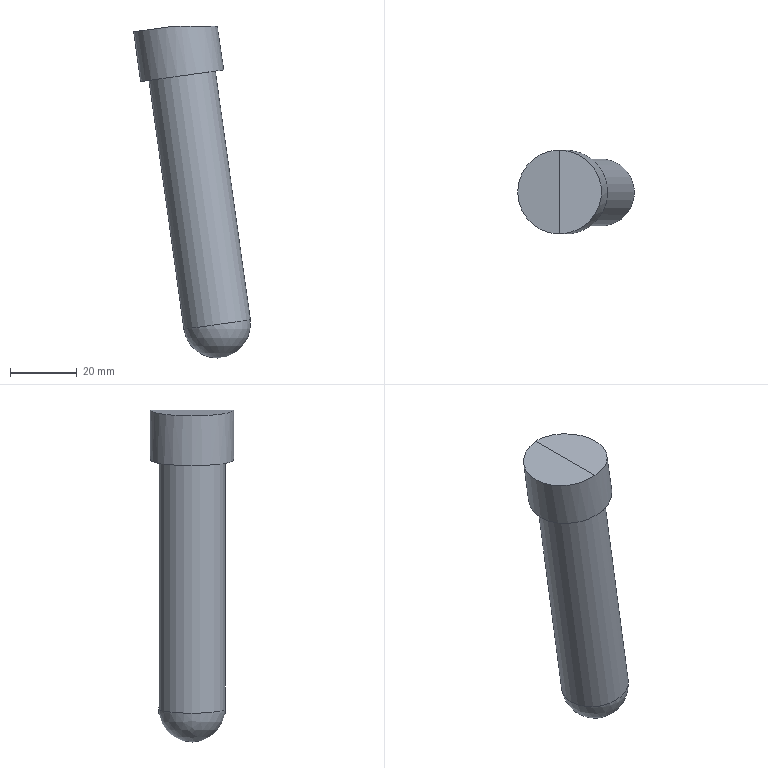Part | STEP file | P011002S002-011 | 1 solid | 6 faces | box 34.904 x 25 x 99.124 mm | volume 32836 mm3 | plane 3 | cylinder 2 | sphere 1 | commonest cylinder face diameters 20 x1 25 x1
STEP:
#1=CARTESIAN_POINT('',(0.,0.,0.));
#2=DIRECTION('',(0.,0.,1.));
#3=DIRECTION('',(1.,0.,0.));
#4=AXIS2_PLACEMENT_3D('',#1,#2,#3);
#5=CARTESIAN_POINT('',(193.,47.5,61.));
#6=VERTEX_POINT('',#5);
#7=CARTESIAN_POINT('',(193.,72.5,61.));
#8=VERTEX_POINT('',#7);
#9=CARTESIAN_POINT('',(193.,60.,61.));
#10=DIRECTION('',(0.,1.,0.));
#11=VECTOR('',#10,1.);
#12=LINE('',#9,#11);
#13=CARTESIAN_POINT('',(193.,60.,61.));
#14=DIRECTION('',(0.1392,0.,-0.9903));
#15=DIRECTION('',(0.9903,0.,0.1392));
#16=AXIS2_PLACEMENT_3D('',#13,#14,#15);
#17=PLANE('',#16);
#18=CARTESIAN_POINT('',(0.,0.));
#19=DIRECTION('',(0.,-1.));
#20=VECTOR('',#19,1.);
#21=LINE('',#18,#20);
#22=(GEOMETRIC_REPRESENTATION_CONTEXT(2)PARAMETRIC_REPRESENTATION_CONTEXT()REPRESENTATION_CONTEXT('',''));
#23=DEFINITIONAL_REPRESENTATION('',(#21),#22);
#24=PCURVE('',#17,#23);
#25=CARTESIAN_POINT('',(250.,10.,61.));
#26=DIRECTION('',(0.,0.,1.));
#27=DIRECTION('',(-1.,0.,0.));
#28=AXIS2_PLACEMENT_3D('',#25,#26,#27);
#29=PLANE('',#28);
#30=CARTESIAN_POINT('',(57.,-50.));
#31=DIRECTION('',(0.,-1.));
#32=VECTOR('',#31,1.);
#33=LINE('',#30,#32);
#34=(GEOMETRIC_REPRESENTATION_CONTEXT(2)PARAMETRIC_REPRESENTATION_CONTEXT()REPRESENTATION_CONTEXT('',''));
#35=DEFINITIONAL_REPRESENTATION('',(#33),#34);
#36=PCURVE('',#29,#35);
#37=SURFACE_CURVE('',#12,(#24,#36),.PCURVE_S1.);
#38=EDGE_CURVE('',#6,#8,#37,.T.);
#39=ORIENTED_EDGE('',*,*,#38,.T.);
#40=CARTESIAN_POINT('',(180.622,60.,59.26));
#41=VERTEX_POINT('',#40);
#42=CARTESIAN_POINT('',(193.,60.,61.));
#43=DIRECTION('',(-0.1392,0.,0.9903));
#44=DIRECTION('',(0.9903,0.,0.1392));
#45=AXIS2_PLACEMENT_3D('',#42,#43,#44);
#46=CIRCLE('',#45,12.5);
#47=CARTESIAN_POINT('',(12.5,0.));
#48=CARTESIAN_POINT('',(12.5,-21.651));
#49=CARTESIAN_POINT('',(-6.25,-10.825));
#50=CARTESIAN_POINT('',(-25.,0.));
#51=CARTESIAN_POINT('',(-6.25,10.825));
#52=CARTESIAN_POINT('',(12.5,21.651));
#53=CARTESIAN_POINT('',(12.5,0.));
#54=(BOUNDED_CURVE()B_SPLINE_CURVE(2,(#47,#48,#49,#50,#51,#52,#53),.UNSPECIFIED.,.T.,.F.)B_SPLINE_CURVE_WITH_KNOTS((1,2,2,2,2,1),(-2.094,0.,2.094,4.189,6.283,8.378),.UNSPECIFIED.)CURVE()GEOMETRIC_REPRESENTATION_ITEM()RATIONAL_B_SPLINE_CURVE((1.,0.5,1.,0.5,1.,0.5,1.))REPRESENTATION_ITEM(''));
#55=(GEOMETRIC_REPRESENTATION_CONTEXT(2)PARAMETRIC_REPRESENTATION_CONTEXT()REPRESENTATION_CONTEXT('',''));
#56=DEFINITIONAL_REPRESENTATION('',(#54),#55);
#57=PCURVE('',#17,#56);
#58=CARTESIAN_POINT('',(223.831,60.,-158.375));
#59=DIRECTION('',(-0.1392,0.,0.9903));
#60=DIRECTION('',(-0.9903,0.,-0.1392));
#61=AXIS2_PLACEMENT_3D('',#58,#59,#60);
#62=CYLINDRICAL_SURFACE('',#61,12.5);
#63=CARTESIAN_POINT('',(3.142,221.531));
#64=DIRECTION('',(1.,0.));
#65=VECTOR('',#64,1.);
#66=LINE('',#63,#65);
#67=(GEOMETRIC_REPRESENTATION_CONTEXT(2)PARAMETRIC_REPRESENTATION_CONTEXT()REPRESENTATION_CONTEXT('',''));
#68=DEFINITIONAL_REPRESENTATION('',(#66),#67);
#69=PCURVE('',#62,#68);
#70=SURFACE_CURVE('',#46,(#57,#69),.PCURVE_S1.);
#71=EDGE_CURVE('',#8,#41,#70,.T.);
#72=ORIENTED_EDGE('',*,*,#71,.T.);
#73=CARTESIAN_POINT('',(193.,60.,61.));
#74=DIRECTION('',(-0.1392,0.,0.9903));
#75=DIRECTION('',(0.9903,0.,0.1392));
#76=AXIS2_PLACEMENT_3D('',#73,#74,#75);
#77=CIRCLE('',#76,12.5);
#78=CARTESIAN_POINT('',(12.5,0.));
#79=CARTESIAN_POINT('',(12.5,-21.651));
#80=CARTESIAN_POINT('',(-6.25,-10.825));
#81=CARTESIAN_POINT('',(-25.,0.));
#82=CARTESIAN_POINT('',(-6.25,10.825));
#83=CARTESIAN_POINT('',(12.5,21.651));
#84=CARTESIAN_POINT('',(12.5,0.));
#85=(BOUNDED_CURVE()B_SPLINE_CURVE(2,(#78,#79,#80,#81,#82,#83,#84),.UNSPECIFIED.,.T.,.F.)B_SPLINE_CURVE_WITH_KNOTS((1,2,2,2,2,1),(-2.094,0.,2.094,4.189,6.283,8.378),.UNSPECIFIED.)CURVE()GEOMETRIC_REPRESENTATION_ITEM()RATIONAL_B_SPLINE_CURVE((1.,0.5,1.,0.5,1.,0.5,1.))REPRESENTATION_ITEM(''));
#86=(GEOMETRIC_REPRESENTATION_CONTEXT(2)PARAMETRIC_REPRESENTATION_CONTEXT()REPRESENTATION_CONTEXT('',''));
#87=DEFINITIONAL_REPRESENTATION('',(#85),#86);
#88=PCURVE('',#17,#87);
#89=CARTESIAN_POINT('',(-3.142,221.531));
#90=DIRECTION('',(1.,0.));
#91=VECTOR('',#90,1.);
#92=LINE('',#89,#91);
#93=(GEOMETRIC_REPRESENTATION_CONTEXT(2)PARAMETRIC_REPRESENTATION_CONTEXT()REPRESENTATION_CONTEXT('',''));
#94=DEFINITIONAL_REPRESENTATION('',(#92),#93);
#95=PCURVE('',#62,#94);
#96=SURFACE_CURVE('',#77,(#88,#95),.PCURVE_S1.);
#97=EDGE_CURVE('',#41,#6,#96,.T.);
#98=ORIENTED_EDGE('',*,*,#97,.T.);
#99=EDGE_LOOP('',(#39,#72,#98));
#100=FACE_BOUND('',#99,.T.);
#101=ADVANCED_FACE('',(#100),#17,.F.);
#102=CARTESIAN_POINT('',(182.709,60.,44.406));
#103=VERTEX_POINT('',#102);
#104=CARTESIAN_POINT('',(195.088,60.,46.146));
#105=DIRECTION('',(0.1392,0.,-0.9903));
#106=DIRECTION('',(-0.9903,0.,-0.1392));
#107=AXIS2_PLACEMENT_3D('',#104,#105,#106);
#108=CIRCLE('',#107,12.5);
#109=CARTESIAN_POINT('',(6.283,206.531));
#110=DIRECTION('',(-1.,0.));
#111=VECTOR('',#110,1.);
#112=LINE('',#109,#111);
#113=(GEOMETRIC_REPRESENTATION_CONTEXT(2)PARAMETRIC_REPRESENTATION_CONTEXT()REPRESENTATION_CONTEXT('',''));
#114=DEFINITIONAL_REPRESENTATION('',(#112),#113);
#115=PCURVE('',#62,#114);
#116=CARTESIAN_POINT('',(195.088,105.,46.146));
#117=DIRECTION('',(-0.1392,0.,0.9903));
#118=DIRECTION('',(-0.9903,0.,-0.1392));
#119=AXIS2_PLACEMENT_3D('',#116,#117,#118);
#120=PLANE('',#119);
#121=CARTESIAN_POINT('',(12.5,45.));
#122=CARTESIAN_POINT('',(12.5,23.349));
#123=CARTESIAN_POINT('',(-6.25,34.175));
#124=CARTESIAN_POINT('',(-25.,45.));
#125=CARTESIAN_POINT('',(-6.25,55.825));
#126=CARTESIAN_POINT('',(12.5,66.651));
#127=CARTESIAN_POINT('',(12.5,45.));
#128=(BOUNDED_CURVE()B_SPLINE_CURVE(2,(#121,#122,#123,#124,#125,#126,#127),.UNSPECIFIED.,.T.,.F.)B_SPLINE_CURVE_WITH_KNOTS((1,2,2,2,2,1),(-2.094,0.,2.094,4.189,6.283,8.378),.UNSPECIFIED.)CURVE()GEOMETRIC_REPRESENTATION_ITEM()RATIONAL_B_SPLINE_CURVE((1.,0.5,1.,0.5,1.,0.5,1.))REPRESENTATION_ITEM(''));
#129=(GEOMETRIC_REPRESENTATION_CONTEXT(2)PARAMETRIC_REPRESENTATION_CONTEXT()REPRESENTATION_CONTEXT('',''));
#130=DEFINITIONAL_REPRESENTATION('',(#128),#129);
#131=PCURVE('',#120,#130);
#132=SURFACE_CURVE('',#108,(#115,#131),.PCURVE_S1.);
#133=EDGE_CURVE('',#103,#103,#132,.T.);
#134=ORIENTED_EDGE('',*,*,#133,.F.);
#135=CARTESIAN_POINT('',(182.709,60.,44.406));
#136=CARTESIAN_POINT('',(180.622,60.,59.26));
#137=B_SPLINE_CURVE_WITH_KNOTS('',1,(#135,#136),.UNSPECIFIED.,.F.,.F.,(2,2),(206.531,221.531),.PIECEWISE_BEZIER_KNOTS.);
#138=CARTESIAN_POINT('',(6.283,0.));
#139=DIRECTION('',(0.,1.));
#140=VECTOR('',#139,1.);
#141=LINE('',#138,#140);
#142=(GEOMETRIC_REPRESENTATION_CONTEXT(2)PARAMETRIC_REPRESENTATION_CONTEXT()REPRESENTATION_CONTEXT('',''));
#143=DEFINITIONAL_REPRESENTATION('',(#141),#142);
#144=PCURVE('',#62,#143);
#145=CARTESIAN_POINT('',(0.,0.));
#146=DIRECTION('',(0.,1.));
#147=VECTOR('',#146,1.);
#148=LINE('',#145,#147);
#149=(GEOMETRIC_REPRESENTATION_CONTEXT(2)PARAMETRIC_REPRESENTATION_CONTEXT()REPRESENTATION_CONTEXT('',''));
#150=DEFINITIONAL_REPRESENTATION('',(#148),#149);
#151=PCURVE('',#62,#150);
#152=SEAM_CURVE('',#137,(#144,#151),.PCURVE_S1.);
#153=EDGE_CURVE('',#103,#41,#152,.T.);
#154=ORIENTED_EDGE('',*,*,#153,.T.);
#155=ORIENTED_EDGE('',*,*,#71,.F.);
#156=CARTESIAN_POINT('',(193.,60.,61.));
#157=DIRECTION('',(0.,0.,-1.));
#158=DIRECTION('',(-1.,0.,0.));
#159=AXIS2_PLACEMENT_3D('',#156,#157,#158);
#160=ELLIPSE('',#159,12.623,12.5);
#161=CARTESIAN_POINT('',(4.712,221.531));
#162=CARTESIAN_POINT('',(4.665,221.447));
#163=CARTESIAN_POINT('',(4.57,221.28));
#164=CARTESIAN_POINT('',(4.427,221.034));
#165=CARTESIAN_POINT('',(4.284,220.799));
#166=CARTESIAN_POINT('',(4.141,220.578));
#167=CARTESIAN_POINT('',(3.998,220.377));
#168=CARTESIAN_POINT('',(3.856,220.199));
#169=CARTESIAN_POINT('',(3.713,220.048));
#170=CARTESIAN_POINT('',(3.57,219.928));
#171=CARTESIAN_POINT('',(3.427,219.84));
#172=CARTESIAN_POINT('',(3.284,219.786));
#173=CARTESIAN_POINT('',(3.142,219.768));
#174=CARTESIAN_POINT('',(2.999,219.786));
#175=CARTESIAN_POINT('',(2.856,219.84));
#176=CARTESIAN_POINT('',(2.713,219.928));
#177=CARTESIAN_POINT('',(2.57,220.048));
#178=CARTESIAN_POINT('',(2.428,220.199));
#179=CARTESIAN_POINT('',(2.285,220.377));
#180=CARTESIAN_POINT('',(2.142,220.578));
#181=CARTESIAN_POINT('',(1.999,220.799));
#182=CARTESIAN_POINT('',(1.856,221.034));
#183=CARTESIAN_POINT('',(1.714,221.28));
#184=CARTESIAN_POINT('',(1.618,221.447));
#185=CARTESIAN_POINT('',(1.571,221.531));
#186=B_SPLINE_CURVE_WITH_KNOTS('',3,(#161,#162,#163,#164,#165,#166,#167,#168,#169,#170,#171,#172,#173,#174,#175,#176,#177,#178,#179,#180,#181,#182,#183,#184,#185),.UNSPECIFIED.,.F.,.F.,(4,1,1,1,1,1,1,1,1,1,1,1,1,1,1,1,1,1,1,1,1,1,4),(1.571,1.714,1.856,1.999,2.142,2.285,2.428,2.57,2.713,2.856,2.999,3.142,3.284,3.427,3.57,3.713,3.856,3.998,4.141,4.284,4.427,4.57,4.712),.QUASI_UNIFORM_KNOTS.);
#187=(GEOMETRIC_REPRESENTATION_CONTEXT(2)PARAMETRIC_REPRESENTATION_CONTEXT()REPRESENTATION_CONTEXT('',''));
#188=DEFINITIONAL_REPRESENTATION('',(#186),#187);
#189=PCURVE('',#62,#188);
#190=CARTESIAN_POINT('',(69.623,-50.));
#191=CARTESIAN_POINT('',(69.623,-71.651));
#192=CARTESIAN_POINT('',(50.689,-60.825));
#193=CARTESIAN_POINT('',(31.754,-50.));
#194=CARTESIAN_POINT('',(50.689,-39.175));
#195=CARTESIAN_POINT('',(69.623,-28.349));
#196=CARTESIAN_POINT('',(69.623,-50.));
#197=(BOUNDED_CURVE()B_SPLINE_CURVE(2,(#190,#191,#192,#193,#194,#195,#196),.UNSPECIFIED.,.T.,.F.)B_SPLINE_CURVE_WITH_KNOTS((1,2,2,2,2,1),(-2.094,0.,2.094,4.189,6.283,8.378),.UNSPECIFIED.)CURVE()GEOMETRIC_REPRESENTATION_ITEM()RATIONAL_B_SPLINE_CURVE((1.,0.5,1.,0.5,1.,0.5,1.))REPRESENTATION_ITEM(''));
#198=(GEOMETRIC_REPRESENTATION_CONTEXT(2)PARAMETRIC_REPRESENTATION_CONTEXT()REPRESENTATION_CONTEXT('',''));
#199=DEFINITIONAL_REPRESENTATION('',(#197),#198);
#200=PCURVE('',#29,#199);
#201=SURFACE_CURVE('',#160,(#189,#200),.PCURVE_S1.);
#202=EDGE_CURVE('',#8,#6,#201,.T.);
#203=ORIENTED_EDGE('',*,*,#202,.T.);
#204=ORIENTED_EDGE('',*,*,#97,.F.);
#205=ORIENTED_EDGE('',*,*,#153,.F.);
#206=EDGE_LOOP('',(#134,#154,#155,#203,#204,#205));
#207=FACE_BOUND('',#206,.T.);
#208=ADVANCED_FACE('',(#207),#62,.T.);
#209=CARTESIAN_POINT('',(195.623,60.,-29.516));
#210=VERTEX_POINT('',#209);
#211=CARTESIAN_POINT('',(205.526,60.,-28.124));
#212=DIRECTION('',(0.1392,0.,-0.9903));
#213=DIRECTION('',(-0.9903,0.,-0.1392));
#214=AXIS2_PLACEMENT_3D('',#211,#212,#213);
#215=CIRCLE('',#214,10.);
#216=CARTESIAN_POINT('',(223.831,60.,-158.375));
#217=DIRECTION('',(-0.1392,0.,0.9903));
#218=DIRECTION('',(-0.9903,0.,-0.1392));
#219=AXIS2_PLACEMENT_3D('',#216,#217,#218);
#220=CYLINDRICAL_SURFACE('',#219,10.);
#221=CARTESIAN_POINT('',(6.283,131.531));
#222=DIRECTION('',(-1.,0.));
#223=VECTOR('',#222,1.);
#224=LINE('',#221,#223);
#225=(GEOMETRIC_REPRESENTATION_CONTEXT(2)PARAMETRIC_REPRESENTATION_CONTEXT()REPRESENTATION_CONTEXT('',''));
#226=DEFINITIONAL_REPRESENTATION('',(#224),#225);
#227=PCURVE('',#220,#226);
#228=CARTESIAN_POINT('',(205.526,60.,-28.124));
#229=DIRECTION('',(0.,0.,1.));
#230=DIRECTION('',(-1.,0.,0.));
#231=AXIS2_PLACEMENT_3D('',#228,#229,#230);
#232=SPHERICAL_SURFACE('',#231,10.);
#233=CARTESIAN_POINT('',(6.283,-0.1396));
#234=CARTESIAN_POINT('',(6.187,-0.1397));
#235=CARTESIAN_POINT('',(5.995,-0.1357));
#236=CARTESIAN_POINT('',(5.707,-0.119));
#237=CARTESIAN_POINT('',(5.421,-0.0925));
#238=CARTESIAN_POINT('',(5.137,-0.05863));
#239=CARTESIAN_POINT('',(4.854,-0.02007));
#240=CARTESIAN_POINT('',(4.571,0.02007));
#241=CARTESIAN_POINT('',(4.288,0.05863));
#242=CARTESIAN_POINT('',(4.003,0.0925));
#243=CARTESIAN_POINT('',(3.717,0.119));
#244=CARTESIAN_POINT('',(3.43,0.1358));
#245=CARTESIAN_POINT('',(3.142,0.1416));
#246=CARTESIAN_POINT('',(2.853,0.1358));
#247=CARTESIAN_POINT('',(2.566,0.119));
#248=CARTESIAN_POINT('',(2.28,0.0925));
#249=CARTESIAN_POINT('',(1.995,0.05863));
#250=CARTESIAN_POINT('',(1.712,0.02007));
#251=CARTESIAN_POINT('',(1.429,-0.02007));
#252=CARTESIAN_POINT('',(1.146,-0.05863));
#253=CARTESIAN_POINT('',(0.8619,-0.0925));
#254=CARTESIAN_POINT('',(0.5759,-0.119));
#255=CARTESIAN_POINT('',(0.2884,-0.1357));
#256=CARTESIAN_POINT('',(0.09616,-0.1397));
#257=CARTESIAN_POINT('',(0.,-0.1396));
#258=B_SPLINE_CURVE_WITH_KNOTS('',3,(#233,#234,#235,#236,#237,#238,#239,#240,#241,#242,#243,#244,#245,#246,#247,#248,#249,#250,#251,#252,#253,#254,#255,#256,#257),.UNSPECIFIED.,.F.,.F.,(4,1,1,1,1,1,1,1,1,1,1,1,1,1,1,1,1,1,1,1,1,1,4),(0.,0.2856,0.5712,0.8568,1.142,1.428,1.714,1.999,2.285,2.57,2.856,3.142,3.427,3.713,3.998,4.284,4.57,4.855,5.141,5.426,5.712,5.998,6.283),.QUASI_UNIFORM_KNOTS.);
#259=(GEOMETRIC_REPRESENTATION_CONTEXT(2)PARAMETRIC_REPRESENTATION_CONTEXT()REPRESENTATION_CONTEXT('',''));
#260=DEFINITIONAL_REPRESENTATION('',(#258),#259);
#261=PCURVE('',#232,#260);
#262=SURFACE_CURVE('',#215,(#227,#261),.PCURVE_S1.);
#263=EDGE_CURVE('',#210,#210,#262,.T.);
#264=ORIENTED_EDGE('',*,*,#263,.F.);
#265=CARTESIAN_POINT('',(185.185,60.,44.754));
#266=VERTEX_POINT('',#265);
#267=CARTESIAN_POINT('',(195.623,60.,-29.516));
#268=CARTESIAN_POINT('',(185.185,60.,44.754));
#269=B_SPLINE_CURVE_WITH_KNOTS('',1,(#267,#268),.UNSPECIFIED.,.F.,.F.,(2,2),(131.531,206.531),.PIECEWISE_BEZIER_KNOTS.);
#270=CARTESIAN_POINT('',(6.283,0.));
#271=DIRECTION('',(0.,1.));
#272=VECTOR('',#271,1.);
#273=LINE('',#270,#272);
#274=(GEOMETRIC_REPRESENTATION_CONTEXT(2)PARAMETRIC_REPRESENTATION_CONTEXT()REPRESENTATION_CONTEXT('',''));
#275=DEFINITIONAL_REPRESENTATION('',(#273),#274);
#276=PCURVE('',#220,#275);
#277=CARTESIAN_POINT('',(0.,0.));
#278=DIRECTION('',(0.,1.));
#279=VECTOR('',#278,1.);
#280=LINE('',#277,#279);
#281=(GEOMETRIC_REPRESENTATION_CONTEXT(2)PARAMETRIC_REPRESENTATION_CONTEXT()REPRESENTATION_CONTEXT('',''));
#282=DEFINITIONAL_REPRESENTATION('',(#280),#281);
#283=PCURVE('',#220,#282);
#284=SEAM_CURVE('',#269,(#276,#283),.PCURVE_S1.);
#285=EDGE_CURVE('',#210,#266,#284,.T.);
#286=ORIENTED_EDGE('',*,*,#285,.T.);
#287=CARTESIAN_POINT('',(195.088,60.,46.146));
#288=DIRECTION('',(0.1392,0.,-0.9903));
#289=DIRECTION('',(-0.9903,0.,-0.1392));
#290=AXIS2_PLACEMENT_3D('',#287,#288,#289);
#291=CIRCLE('',#290,10.);
#292=CARTESIAN_POINT('',(6.283,206.531));
#293=DIRECTION('',(-1.,0.));
#294=VECTOR('',#293,1.);
#295=LINE('',#292,#294);
#296=(GEOMETRIC_REPRESENTATION_CONTEXT(2)PARAMETRIC_REPRESENTATION_CONTEXT()REPRESENTATION_CONTEXT('',''));
#297=DEFINITIONAL_REPRESENTATION('',(#295),#296);
#298=PCURVE('',#220,#297);
#299=CARTESIAN_POINT('',(10.,45.));
#300=CARTESIAN_POINT('',(10.,27.679));
#301=CARTESIAN_POINT('',(-5.,36.34));
#302=CARTESIAN_POINT('',(-20.,45.));
#303=CARTESIAN_POINT('',(-5.,53.66));
#304=CARTESIAN_POINT('',(10.,62.321));
#305=CARTESIAN_POINT('',(10.,45.));
#306=(BOUNDED_CURVE()B_SPLINE_CURVE(2,(#299,#300,#301,#302,#303,#304,#305),.UNSPECIFIED.,.T.,.F.)B_SPLINE_CURVE_WITH_KNOTS((1,2,2,2,2,1),(-2.094,0.,2.094,4.189,6.283,8.378),.UNSPECIFIED.)CURVE()GEOMETRIC_REPRESENTATION_ITEM()RATIONAL_B_SPLINE_CURVE((1.,0.5,1.,0.5,1.,0.5,1.))REPRESENTATION_ITEM(''));
#307=(GEOMETRIC_REPRESENTATION_CONTEXT(2)PARAMETRIC_REPRESENTATION_CONTEXT()REPRESENTATION_CONTEXT('',''));
#308=DEFINITIONAL_REPRESENTATION('',(#306),#307);
#309=PCURVE('',#120,#308);
#310=SURFACE_CURVE('',#291,(#298,#309),.PCURVE_S1.);
#311=EDGE_CURVE('',#266,#266,#310,.T.);
#312=ORIENTED_EDGE('',*,*,#311,.T.);
#313=ORIENTED_EDGE('',*,*,#285,.F.);
#314=EDGE_LOOP('',(#264,#286,#312,#313));
#315=FACE_BOUND('',#314,.T.);
#316=ADVANCED_FACE('',(#315),#220,.T.);
#317=ORIENTED_EDGE('',*,*,#133,.T.);
#318=EDGE_LOOP('',(#317));
#319=FACE_BOUND('',#318,.T.);
#320=ORIENTED_EDGE('',*,*,#311,.F.);
#321=EDGE_LOOP('',(#320));
#322=FACE_BOUND('',#321,.T.);
#323=ADVANCED_FACE('',(#319,#322),#120,.F.);
#324=ORIENTED_EDGE('',*,*,#263,.T.);
#325=CARTESIAN_POINT('',(205.526,60.,-38.124));
#326=VERTEX_POINT('',#325);
#327=CARTESIAN_POINT('',(205.526,60.,-38.124));
#328=CARTESIAN_POINT('',(203.14,60.,-38.124));
#329=CARTESIAN_POINT('',(200.755,60.,-37.441));
#330=CARTESIAN_POINT('',(198.614,60.,-36.076));
#331=CARTESIAN_POINT('',(196.963,60.,-34.145));
#332=CARTESIAN_POINT('',(195.955,60.,-31.878));
#333=CARTESIAN_POINT('',(195.623,60.,-29.516));
#334=B_SPLINE_CURVE_WITH_KNOTS('',6,(#327,#328,#329,#330,#331,#332,#333),.UNSPECIFIED.,.F.,.F.,(7,7),(-1.571,-0.1396),.PIECEWISE_BEZIER_KNOTS.);
#335=CARTESIAN_POINT('',(0.,0.));
#336=DIRECTION('',(0.,1.));
#337=VECTOR('',#336,1.);
#338=LINE('',#335,#337);
#339=(GEOMETRIC_REPRESENTATION_CONTEXT(2)PARAMETRIC_REPRESENTATION_CONTEXT()REPRESENTATION_CONTEXT('',''));
#340=DEFINITIONAL_REPRESENTATION('',(#338),#339);
#341=PCURVE('',#232,#340);
#342=CARTESIAN_POINT('',(6.283,0.));
#343=DIRECTION('',(0.,1.));
#344=VECTOR('',#343,1.);
#345=LINE('',#342,#344);
#346=(GEOMETRIC_REPRESENTATION_CONTEXT(2)PARAMETRIC_REPRESENTATION_CONTEXT()REPRESENTATION_CONTEXT('',''));
#347=DEFINITIONAL_REPRESENTATION('',(#345),#346);
#348=PCURVE('',#232,#347);
#349=SEAM_CURVE('',#334,(#341,#348),.PCURVE_S1.);
#350=EDGE_CURVE('',#326,#210,#349,.T.);
#351=ORIENTED_EDGE('',*,*,#350,.F.);
#352=ORIENTED_EDGE('',*,*,#350,.T.);
#353=EDGE_LOOP('',(#324,#351,#352));
#354=FACE_BOUND('',#353,.T.);
#355=ADVANCED_FACE('',(#354),#232,.T.);
#356=ORIENTED_EDGE('',*,*,#202,.F.);
#357=ORIENTED_EDGE('',*,*,#38,.F.);
#358=EDGE_LOOP('',(#356,#357));
#359=FACE_BOUND('',#358,.T.);
#360=ADVANCED_FACE('',(#359),#29,.T.);
#361=CLOSED_SHELL('',(#101,#208,#316,#323,#355,#360));
#362=MANIFOLD_SOLID_BREP('',#361);
#363=(LENGTH_UNIT()NAMED_UNIT(*)SI_UNIT(.MILLI.,.METRE.));
#364=UNCERTAINTY_MEASURE_WITH_UNIT(LENGTH_MEASURE(0.000005),#363,'','');
#365=(NAMED_UNIT(*)PLANE_ANGLE_UNIT()SI_UNIT($,.RADIAN.));
#366=(NAMED_UNIT(*)SI_UNIT($,.STERADIAN.)SOLID_ANGLE_UNIT());
#367=(GEOMETRIC_REPRESENTATION_CONTEXT(3)GLOBAL_UNCERTAINTY_ASSIGNED_CONTEXT((#364))GLOBAL_UNIT_ASSIGNED_CONTEXT((#363,#365,#366))REPRESENTATION_CONTEXT('',''));
#368=ADVANCED_BREP_SHAPE_REPRESENTATION('',(#4,#362),#367);